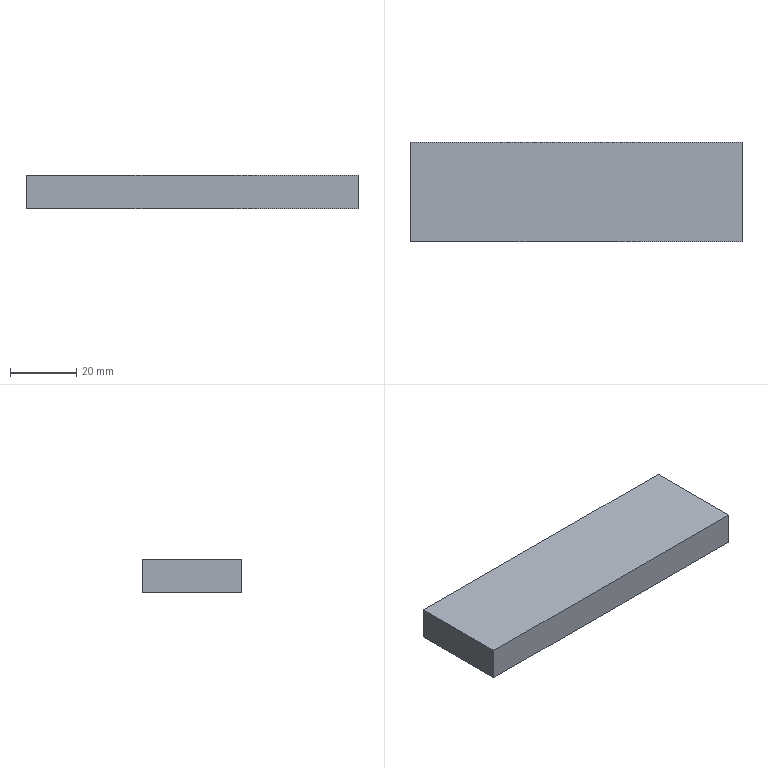Part | STEP file | 04-Travel stopper | 1 solid | 6 faces | box 100 x 30 x 10 mm | volume 30000 mm3 | plane 6
STEP:
#1=CARTESIAN_POINT('',(0.,0.,0.));
#2=DIRECTION('',(0.,0.,1.));
#3=DIRECTION('',(1.,0.,0.));
#4=AXIS2_PLACEMENT_3D('',#1,#2,#3);
#5=CARTESIAN_POINT('',(0.,0.,0.));
#6=VERTEX_POINT('',#5);
#7=CARTESIAN_POINT('',(0.,-30.,0.));
#8=VERTEX_POINT('',#7);
#9=CARTESIAN_POINT('',(0.,0.,0.));
#10=DIRECTION('',(0.,-1.,0.));
#11=VECTOR('',#10,1.);
#12=LINE('',#9,#11);
#13=CARTESIAN_POINT('',(0.,0.,10.));
#14=DIRECTION('',(1.,0.,0.));
#15=DIRECTION('',(0.,1.,0.));
#16=AXIS2_PLACEMENT_3D('',#13,#14,#15);
#17=PLANE('',#16);
#18=CARTESIAN_POINT('',(0.,-10.));
#19=DIRECTION('',(-1.,0.));
#20=VECTOR('',#19,1.);
#21=LINE('',#18,#20);
#22=(GEOMETRIC_REPRESENTATION_CONTEXT(2)PARAMETRIC_REPRESENTATION_CONTEXT()REPRESENTATION_CONTEXT('',''));
#23=DEFINITIONAL_REPRESENTATION('',(#21),#22);
#24=PCURVE('',#17,#23);
#25=CARTESIAN_POINT('',(0.,0.,0.));
#26=DIRECTION('',(0.,0.,1.));
#27=DIRECTION('',(1.,0.,0.));
#28=AXIS2_PLACEMENT_3D('',#25,#26,#27);
#29=PLANE('',#28);
#30=CARTESIAN_POINT('',(0.,0.));
#31=DIRECTION('',(0.,-1.));
#32=VECTOR('',#31,1.);
#33=LINE('',#30,#32);
#34=(GEOMETRIC_REPRESENTATION_CONTEXT(2)PARAMETRIC_REPRESENTATION_CONTEXT()REPRESENTATION_CONTEXT('',''));
#35=DEFINITIONAL_REPRESENTATION('',(#33),#34);
#36=PCURVE('',#29,#35);
#37=SURFACE_CURVE('',#12,(#24,#36),.PCURVE_S1.);
#38=EDGE_CURVE('',#6,#8,#37,.T.);
#39=ORIENTED_EDGE('',*,*,#38,.T.);
#40=CARTESIAN_POINT('',(0.,-30.,10.));
#41=VERTEX_POINT('',#40);
#42=CARTESIAN_POINT('',(0.,-30.,10.));
#43=DIRECTION('',(0.,0.,-1.));
#44=VECTOR('',#43,1.);
#45=LINE('',#42,#44);
#46=CARTESIAN_POINT('',(-30.,0.));
#47=DIRECTION('',(0.,-1.));
#48=VECTOR('',#47,1.);
#49=LINE('',#46,#48);
#50=(GEOMETRIC_REPRESENTATION_CONTEXT(2)PARAMETRIC_REPRESENTATION_CONTEXT()REPRESENTATION_CONTEXT('',''));
#51=DEFINITIONAL_REPRESENTATION('',(#49),#50);
#52=PCURVE('',#17,#51);
#53=CARTESIAN_POINT('',(0.,-30.,10.));
#54=DIRECTION('',(0.,1.,0.));
#55=DIRECTION('',(0.,0.,1.));
#56=AXIS2_PLACEMENT_3D('',#53,#54,#55);
#57=PLANE('',#56);
#58=CARTESIAN_POINT('',(0.,0.));
#59=DIRECTION('',(-1.,0.));
#60=VECTOR('',#59,1.);
#61=LINE('',#58,#60);
#62=(GEOMETRIC_REPRESENTATION_CONTEXT(2)PARAMETRIC_REPRESENTATION_CONTEXT()REPRESENTATION_CONTEXT('',''));
#63=DEFINITIONAL_REPRESENTATION('',(#61),#62);
#64=PCURVE('',#57,#63);
#65=SURFACE_CURVE('',#45,(#52,#64),.PCURVE_S1.);
#66=EDGE_CURVE('',#41,#8,#65,.T.);
#67=ORIENTED_EDGE('',*,*,#66,.F.);
#68=CARTESIAN_POINT('',(0.,0.,10.));
#69=VERTEX_POINT('',#68);
#70=CARTESIAN_POINT('',(0.,0.,10.));
#71=DIRECTION('',(0.,-1.,0.));
#72=VECTOR('',#71,1.);
#73=LINE('',#70,#72);
#74=CARTESIAN_POINT('',(0.,0.));
#75=DIRECTION('',(-1.,0.));
#76=VECTOR('',#75,1.);
#77=LINE('',#74,#76);
#78=(GEOMETRIC_REPRESENTATION_CONTEXT(2)PARAMETRIC_REPRESENTATION_CONTEXT()REPRESENTATION_CONTEXT('',''));
#79=DEFINITIONAL_REPRESENTATION('',(#77),#78);
#80=PCURVE('',#17,#79);
#81=CARTESIAN_POINT('',(0.,0.,10.));
#82=DIRECTION('',(0.,0.,1.));
#83=DIRECTION('',(1.,0.,0.));
#84=AXIS2_PLACEMENT_3D('',#81,#82,#83);
#85=PLANE('',#84);
#86=CARTESIAN_POINT('',(0.,0.));
#87=DIRECTION('',(0.,-1.));
#88=VECTOR('',#87,1.);
#89=LINE('',#86,#88);
#90=(GEOMETRIC_REPRESENTATION_CONTEXT(2)PARAMETRIC_REPRESENTATION_CONTEXT()REPRESENTATION_CONTEXT('',''));
#91=DEFINITIONAL_REPRESENTATION('',(#89),#90);
#92=PCURVE('',#85,#91);
#93=SURFACE_CURVE('',#73,(#80,#92),.PCURVE_S1.);
#94=EDGE_CURVE('',#69,#41,#93,.T.);
#95=ORIENTED_EDGE('',*,*,#94,.F.);
#96=CARTESIAN_POINT('',(0.,0.,10.));
#97=DIRECTION('',(0.,0.,-1.));
#98=VECTOR('',#97,1.);
#99=LINE('',#96,#98);
#100=CARTESIAN_POINT('',(0.,0.));
#101=DIRECTION('',(0.,-1.));
#102=VECTOR('',#101,1.);
#103=LINE('',#100,#102);
#104=(GEOMETRIC_REPRESENTATION_CONTEXT(2)PARAMETRIC_REPRESENTATION_CONTEXT()REPRESENTATION_CONTEXT('',''));
#105=DEFINITIONAL_REPRESENTATION('',(#103),#104);
#106=PCURVE('',#17,#105);
#107=CARTESIAN_POINT('',(0.,0.,10.));
#108=DIRECTION('',(0.,-1.,0.));
#109=DIRECTION('',(0.,0.,-1.));
#110=AXIS2_PLACEMENT_3D('',#107,#108,#109);
#111=PLANE('',#110);
#112=CARTESIAN_POINT('',(0.,0.));
#113=DIRECTION('',(1.,0.));
#114=VECTOR('',#113,1.);
#115=LINE('',#112,#114);
#116=(GEOMETRIC_REPRESENTATION_CONTEXT(2)PARAMETRIC_REPRESENTATION_CONTEXT()REPRESENTATION_CONTEXT('',''));
#117=DEFINITIONAL_REPRESENTATION('',(#115),#116);
#118=PCURVE('',#111,#117);
#119=SURFACE_CURVE('',#99,(#106,#118),.PCURVE_S1.);
#120=EDGE_CURVE('',#69,#6,#119,.T.);
#121=ORIENTED_EDGE('',*,*,#120,.T.);
#122=EDGE_LOOP('',(#39,#67,#95,#121));
#123=FACE_BOUND('',#122,.T.);
#124=ADVANCED_FACE('',(#123),#17,.F.);
#125=CARTESIAN_POINT('',(100.,-30.,0.));
#126=VERTEX_POINT('',#125);
#127=CARTESIAN_POINT('',(0.,-30.,0.));
#128=DIRECTION('',(1.,0.,0.));
#129=VECTOR('',#128,1.);
#130=LINE('',#127,#129);
#131=CARTESIAN_POINT('',(-10.,0.));
#132=DIRECTION('',(0.,1.));
#133=VECTOR('',#132,1.);
#134=LINE('',#131,#133);
#135=(GEOMETRIC_REPRESENTATION_CONTEXT(2)PARAMETRIC_REPRESENTATION_CONTEXT()REPRESENTATION_CONTEXT('',''));
#136=DEFINITIONAL_REPRESENTATION('',(#134),#135);
#137=PCURVE('',#57,#136);
#138=CARTESIAN_POINT('',(0.,-30.));
#139=DIRECTION('',(1.,0.));
#140=VECTOR('',#139,1.);
#141=LINE('',#138,#140);
#142=(GEOMETRIC_REPRESENTATION_CONTEXT(2)PARAMETRIC_REPRESENTATION_CONTEXT()REPRESENTATION_CONTEXT('',''));
#143=DEFINITIONAL_REPRESENTATION('',(#141),#142);
#144=PCURVE('',#29,#143);
#145=SURFACE_CURVE('',#130,(#137,#144),.PCURVE_S1.);
#146=EDGE_CURVE('',#8,#126,#145,.T.);
#147=ORIENTED_EDGE('',*,*,#146,.T.);
#148=CARTESIAN_POINT('',(100.,-30.,10.));
#149=VERTEX_POINT('',#148);
#150=CARTESIAN_POINT('',(100.,-30.,10.));
#151=DIRECTION('',(0.,0.,-1.));
#152=VECTOR('',#151,1.);
#153=LINE('',#150,#152);
#154=CARTESIAN_POINT('',(0.,100.));
#155=DIRECTION('',(-1.,0.));
#156=VECTOR('',#155,1.);
#157=LINE('',#154,#156);
#158=(GEOMETRIC_REPRESENTATION_CONTEXT(2)PARAMETRIC_REPRESENTATION_CONTEXT()REPRESENTATION_CONTEXT('',''));
#159=DEFINITIONAL_REPRESENTATION('',(#157),#158);
#160=PCURVE('',#57,#159);
#161=CARTESIAN_POINT('',(100.,0.,10.));
#162=DIRECTION('',(-1.,0.,0.));
#163=DIRECTION('',(0.,0.,1.));
#164=AXIS2_PLACEMENT_3D('',#161,#162,#163);
#165=PLANE('',#164);
#166=CARTESIAN_POINT('',(0.,-30.));
#167=DIRECTION('',(-1.,0.));
#168=VECTOR('',#167,1.);
#169=LINE('',#166,#168);
#170=(GEOMETRIC_REPRESENTATION_CONTEXT(2)PARAMETRIC_REPRESENTATION_CONTEXT()REPRESENTATION_CONTEXT('',''));
#171=DEFINITIONAL_REPRESENTATION('',(#169),#170);
#172=PCURVE('',#165,#171);
#173=SURFACE_CURVE('',#153,(#160,#172),.PCURVE_S1.);
#174=EDGE_CURVE('',#149,#126,#173,.T.);
#175=ORIENTED_EDGE('',*,*,#174,.F.);
#176=CARTESIAN_POINT('',(0.,-30.,10.));
#177=DIRECTION('',(1.,0.,0.));
#178=VECTOR('',#177,1.);
#179=LINE('',#176,#178);
#180=CARTESIAN_POINT('',(0.,0.));
#181=DIRECTION('',(0.,1.));
#182=VECTOR('',#181,1.);
#183=LINE('',#180,#182);
#184=(GEOMETRIC_REPRESENTATION_CONTEXT(2)PARAMETRIC_REPRESENTATION_CONTEXT()REPRESENTATION_CONTEXT('',''));
#185=DEFINITIONAL_REPRESENTATION('',(#183),#184);
#186=PCURVE('',#57,#185);
#187=CARTESIAN_POINT('',(0.,-30.));
#188=DIRECTION('',(1.,0.));
#189=VECTOR('',#188,1.);
#190=LINE('',#187,#189);
#191=(GEOMETRIC_REPRESENTATION_CONTEXT(2)PARAMETRIC_REPRESENTATION_CONTEXT()REPRESENTATION_CONTEXT('',''));
#192=DEFINITIONAL_REPRESENTATION('',(#190),#191);
#193=PCURVE('',#85,#192);
#194=SURFACE_CURVE('',#179,(#186,#193),.PCURVE_S1.);
#195=EDGE_CURVE('',#41,#149,#194,.T.);
#196=ORIENTED_EDGE('',*,*,#195,.F.);
#197=ORIENTED_EDGE('',*,*,#66,.T.);
#198=EDGE_LOOP('',(#147,#175,#196,#197));
#199=FACE_BOUND('',#198,.T.);
#200=ADVANCED_FACE('',(#199),#57,.F.);
#201=CARTESIAN_POINT('',(100.,0.,0.));
#202=VERTEX_POINT('',#201);
#203=CARTESIAN_POINT('',(100.,0.,0.));
#204=DIRECTION('',(0.,1.,0.));
#205=VECTOR('',#204,1.);
#206=LINE('',#203,#205);
#207=CARTESIAN_POINT('',(-10.,0.));
#208=DIRECTION('',(0.,1.));
#209=VECTOR('',#208,1.);
#210=LINE('',#207,#209);
#211=(GEOMETRIC_REPRESENTATION_CONTEXT(2)PARAMETRIC_REPRESENTATION_CONTEXT()REPRESENTATION_CONTEXT('',''));
#212=DEFINITIONAL_REPRESENTATION('',(#210),#211);
#213=PCURVE('',#165,#212);
#214=CARTESIAN_POINT('',(100.,0.));
#215=DIRECTION('',(0.,1.));
#216=VECTOR('',#215,1.);
#217=LINE('',#214,#216);
#218=(GEOMETRIC_REPRESENTATION_CONTEXT(2)PARAMETRIC_REPRESENTATION_CONTEXT()REPRESENTATION_CONTEXT('',''));
#219=DEFINITIONAL_REPRESENTATION('',(#217),#218);
#220=PCURVE('',#29,#219);
#221=SURFACE_CURVE('',#206,(#213,#220),.PCURVE_S1.);
#222=EDGE_CURVE('',#126,#202,#221,.T.);
#223=ORIENTED_EDGE('',*,*,#222,.T.);
#224=CARTESIAN_POINT('',(100.,0.,10.));
#225=VERTEX_POINT('',#224);
#226=CARTESIAN_POINT('',(100.,0.,10.));
#227=DIRECTION('',(0.,0.,-1.));
#228=VECTOR('',#227,1.);
#229=LINE('',#226,#228);
#230=CARTESIAN_POINT('',(0.,0.));
#231=DIRECTION('',(-1.,0.));
#232=VECTOR('',#231,1.);
#233=LINE('',#230,#232);
#234=(GEOMETRIC_REPRESENTATION_CONTEXT(2)PARAMETRIC_REPRESENTATION_CONTEXT()REPRESENTATION_CONTEXT('',''));
#235=DEFINITIONAL_REPRESENTATION('',(#233),#234);
#236=PCURVE('',#165,#235);
#237=CARTESIAN_POINT('',(0.,100.));
#238=DIRECTION('',(1.,0.));
#239=VECTOR('',#238,1.);
#240=LINE('',#237,#239);
#241=(GEOMETRIC_REPRESENTATION_CONTEXT(2)PARAMETRIC_REPRESENTATION_CONTEXT()REPRESENTATION_CONTEXT('',''));
#242=DEFINITIONAL_REPRESENTATION('',(#240),#241);
#243=PCURVE('',#111,#242);
#244=SURFACE_CURVE('',#229,(#236,#243),.PCURVE_S1.);
#245=EDGE_CURVE('',#225,#202,#244,.T.);
#246=ORIENTED_EDGE('',*,*,#245,.F.);
#247=CARTESIAN_POINT('',(100.,0.,10.));
#248=DIRECTION('',(0.,1.,0.));
#249=VECTOR('',#248,1.);
#250=LINE('',#247,#249);
#251=CARTESIAN_POINT('',(0.,0.));
#252=DIRECTION('',(0.,1.));
#253=VECTOR('',#252,1.);
#254=LINE('',#251,#253);
#255=(GEOMETRIC_REPRESENTATION_CONTEXT(2)PARAMETRIC_REPRESENTATION_CONTEXT()REPRESENTATION_CONTEXT('',''));
#256=DEFINITIONAL_REPRESENTATION('',(#254),#255);
#257=PCURVE('',#165,#256);
#258=CARTESIAN_POINT('',(100.,0.));
#259=DIRECTION('',(0.,1.));
#260=VECTOR('',#259,1.);
#261=LINE('',#258,#260);
#262=(GEOMETRIC_REPRESENTATION_CONTEXT(2)PARAMETRIC_REPRESENTATION_CONTEXT()REPRESENTATION_CONTEXT('',''));
#263=DEFINITIONAL_REPRESENTATION('',(#261),#262);
#264=PCURVE('',#85,#263);
#265=SURFACE_CURVE('',#250,(#257,#264),.PCURVE_S1.);
#266=EDGE_CURVE('',#149,#225,#265,.T.);
#267=ORIENTED_EDGE('',*,*,#266,.F.);
#268=ORIENTED_EDGE('',*,*,#174,.T.);
#269=EDGE_LOOP('',(#223,#246,#267,#268));
#270=FACE_BOUND('',#269,.T.);
#271=ADVANCED_FACE('',(#270),#165,.F.);
#272=CARTESIAN_POINT('',(0.,0.,0.));
#273=DIRECTION('',(-1.,0.,0.));
#274=VECTOR('',#273,1.);
#275=LINE('',#272,#274);
#276=CARTESIAN_POINT('',(10.,0.));
#277=DIRECTION('',(0.,-1.));
#278=VECTOR('',#277,1.);
#279=LINE('',#276,#278);
#280=(GEOMETRIC_REPRESENTATION_CONTEXT(2)PARAMETRIC_REPRESENTATION_CONTEXT()REPRESENTATION_CONTEXT('',''));
#281=DEFINITIONAL_REPRESENTATION('',(#279),#280);
#282=PCURVE('',#111,#281);
#283=CARTESIAN_POINT('',(0.,0.));
#284=DIRECTION('',(-1.,0.));
#285=VECTOR('',#284,1.);
#286=LINE('',#283,#285);
#287=(GEOMETRIC_REPRESENTATION_CONTEXT(2)PARAMETRIC_REPRESENTATION_CONTEXT()REPRESENTATION_CONTEXT('',''));
#288=DEFINITIONAL_REPRESENTATION('',(#286),#287);
#289=PCURVE('',#29,#288);
#290=SURFACE_CURVE('',#275,(#282,#289),.PCURVE_S1.);
#291=EDGE_CURVE('',#202,#6,#290,.T.);
#292=ORIENTED_EDGE('',*,*,#291,.T.);
#293=ORIENTED_EDGE('',*,*,#120,.F.);
#294=CARTESIAN_POINT('',(0.,0.,10.));
#295=DIRECTION('',(-1.,0.,0.));
#296=VECTOR('',#295,1.);
#297=LINE('',#294,#296);
#298=CARTESIAN_POINT('',(0.,0.));
#299=DIRECTION('',(0.,-1.));
#300=VECTOR('',#299,1.);
#301=LINE('',#298,#300);
#302=(GEOMETRIC_REPRESENTATION_CONTEXT(2)PARAMETRIC_REPRESENTATION_CONTEXT()REPRESENTATION_CONTEXT('',''));
#303=DEFINITIONAL_REPRESENTATION('',(#301),#302);
#304=PCURVE('',#111,#303);
#305=CARTESIAN_POINT('',(0.,0.));
#306=DIRECTION('',(-1.,0.));
#307=VECTOR('',#306,1.);
#308=LINE('',#305,#307);
#309=(GEOMETRIC_REPRESENTATION_CONTEXT(2)PARAMETRIC_REPRESENTATION_CONTEXT()REPRESENTATION_CONTEXT('',''));
#310=DEFINITIONAL_REPRESENTATION('',(#308),#309);
#311=PCURVE('',#85,#310);
#312=SURFACE_CURVE('',#297,(#304,#311),.PCURVE_S1.);
#313=EDGE_CURVE('',#225,#69,#312,.T.);
#314=ORIENTED_EDGE('',*,*,#313,.F.);
#315=ORIENTED_EDGE('',*,*,#245,.T.);
#316=EDGE_LOOP('',(#292,#293,#314,#315));
#317=FACE_BOUND('',#316,.T.);
#318=ADVANCED_FACE('',(#317),#111,.F.);
#319=ORIENTED_EDGE('',*,*,#94,.T.);
#320=ORIENTED_EDGE('',*,*,#195,.T.);
#321=ORIENTED_EDGE('',*,*,#266,.T.);
#322=ORIENTED_EDGE('',*,*,#313,.T.);
#323=EDGE_LOOP('',(#319,#320,#321,#322));
#324=FACE_BOUND('',#323,.T.);
#325=ADVANCED_FACE('',(#324),#85,.T.);
#326=ORIENTED_EDGE('',*,*,#38,.F.);
#327=ORIENTED_EDGE('',*,*,#291,.F.);
#328=ORIENTED_EDGE('',*,*,#222,.F.);
#329=ORIENTED_EDGE('',*,*,#146,.F.);
#330=EDGE_LOOP('',(#326,#327,#328,#329));
#331=FACE_BOUND('',#330,.T.);
#332=ADVANCED_FACE('',(#331),#29,.F.);
#333=CLOSED_SHELL('',(#124,#200,#271,#318,#325,#332));
#334=MANIFOLD_SOLID_BREP('',#333);
#335=(LENGTH_UNIT()NAMED_UNIT(*)SI_UNIT(.MILLI.,.METRE.));
#336=UNCERTAINTY_MEASURE_WITH_UNIT(LENGTH_MEASURE(0.0000001),#335,'','');
#337=(NAMED_UNIT(*)PLANE_ANGLE_UNIT()SI_UNIT($,.RADIAN.));
#338=(NAMED_UNIT(*)SI_UNIT($,.STERADIAN.)SOLID_ANGLE_UNIT());
#339=(GEOMETRIC_REPRESENTATION_CONTEXT(3)GLOBAL_UNCERTAINTY_ASSIGNED_CONTEXT((#336))GLOBAL_UNIT_ASSIGNED_CONTEXT((#335,#337,#338))REPRESENTATION_CONTEXT('',''));
#340=ADVANCED_BREP_SHAPE_REPRESENTATION('',(#4,#334),#339);